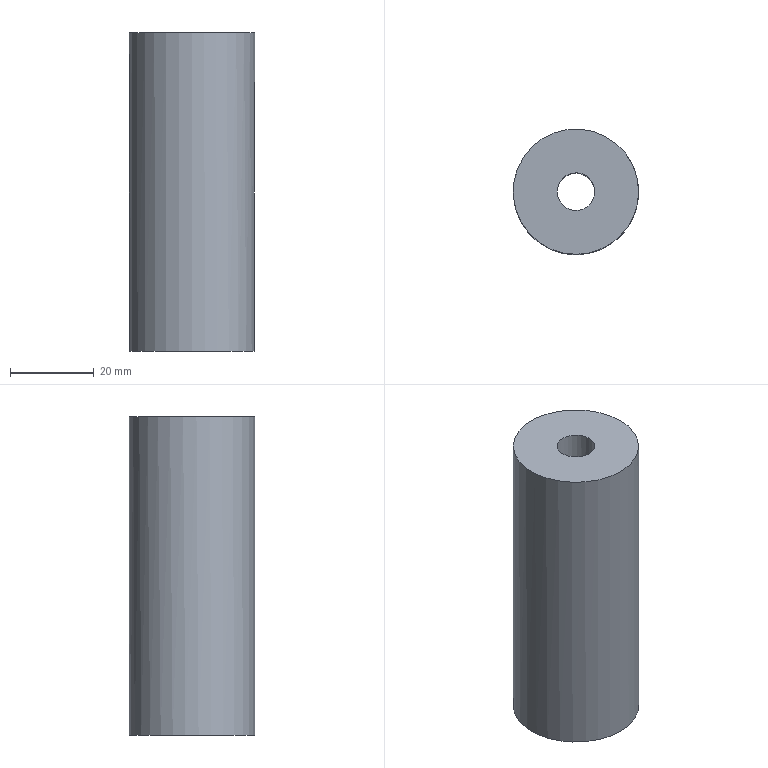Part | NX | features solid 2 | 1 solid | 6 faces | box 30 x 30 x 76.131 mm | volume 47845 mm3 | plane 3 | cylinder 3 | commonest cylinder face diameters 9.007 x1 14.508 x1 30 x1
STEP:
#1=CARTESIAN_POINT('',(797.773,-144.91,104.999));
#2=VERTEX_POINT('',#1);
#3=CARTESIAN_POINT('',(797.773,-129.91,104.999));
#4=DIRECTION('',(-0.000000328,0.000000403,-1.));
#5=DIRECTION('',(0.,-1.,-0.000000403));
#6=AXIS2_PLACEMENT_3D('',#3,#4,#5);
#7=CIRCLE('',#6,15.);
#8=EDGE_CURVE('',#2,#2,#7,.F.);
#9=ORIENTED_EDGE('',*,*,#8,.F.);
#10=EDGE_LOOP('',(#9));
#11=FACE_BOUND('',#10,.T.);
#12=CARTESIAN_POINT('',(796.295,-137.012,104.999));
#13=VERTEX_POINT('',#12);
#14=CARTESIAN_POINT('',(797.773,-129.91,104.999));
#15=DIRECTION('',(-0.000000328,0.000000403,-1.));
#16=DIRECTION('',(-0.2037,-0.979,-0.000000328));
#17=AXIS2_PLACEMENT_3D('',#14,#15,#16);
#18=CIRCLE('',#17,7.254);
#19=EDGE_CURVE('',#13,#13,#18,.F.);
#20=ORIENTED_EDGE('',*,*,#19,.T.);
#21=EDGE_LOOP('',(#20));
#22=FACE_BOUND('',#21,.T.);
#23=CARTESIAN_POINT('',(801.839,-133.976,104.999));
#24=DIRECTION('',(0.000000328,-0.000000403,1.));
#25=DIRECTION('',(-0.7071,-0.7071,-0.000000053));
#26=AXIS2_PLACEMENT_3D('',#23,#24,#25);
#27=PLANE('',#26);
#28=ADVANCED_FACE('',(#11,#22),#27,.F.);
#29=CARTESIAN_POINT('',(812.773,-129.91,181.13));
#30=VERTEX_POINT('',#29);
#31=CARTESIAN_POINT('',(797.773,-129.91,181.13));
#32=DIRECTION('',(0.,0.,-1.));
#33=DIRECTION('',(1.,0.,0.));
#34=AXIS2_PLACEMENT_3D('',#31,#32,#33);
#35=CIRCLE('',#34,15.);
#36=EDGE_CURVE('',#30,#30,#35,.F.);
#37=ORIENTED_EDGE('',*,*,#36,.F.);
#38=EDGE_LOOP('',(#37));
#39=FACE_BOUND('',#38,.T.);
#40=ORIENTED_EDGE('',*,*,#8,.T.);
#41=EDGE_LOOP('',(#40));
#42=FACE_BOUND('',#41,.T.);
#43=CARTESIAN_POINT('',(797.773,-129.91,96.999));
#44=DIRECTION('',(0.000000328,-0.000000403,1.));
#45=DIRECTION('',(-0.2037,-0.979,-0.000000328));
#46=AXIS2_PLACEMENT_3D('',#43,#44,#45);
#47=CYLINDRICAL_SURFACE('',#46,15.);
#48=ADVANCED_FACE('',(#39,#42),#47,.T.);
#49=CARTESIAN_POINT('',(802.276,-129.91,181.13));
#50=VERTEX_POINT('',#49);
#51=CARTESIAN_POINT('',(797.773,-129.91,181.13));
#52=DIRECTION('',(0.,0.,-1.));
#53=DIRECTION('',(1.,0.,0.));
#54=AXIS2_PLACEMENT_3D('',#51,#52,#53);
#55=CIRCLE('',#54,4.503);
#56=EDGE_CURVE('',#50,#50,#55,.T.);
#57=ORIENTED_EDGE('',*,*,#56,.T.);
#58=EDGE_LOOP('',(#57));
#59=FACE_BOUND('',#58,.T.);
#60=ORIENTED_EDGE('',*,*,#36,.T.);
#61=EDGE_LOOP('',(#60));
#62=FACE_BOUND('',#61,.T.);
#63=CARTESIAN_POINT('',(1379.977,36.59,181.13));
#64=DIRECTION('',(0.,0.,-1.));
#65=DIRECTION('',(0.,-1.,0.));
#66=AXIS2_PLACEMENT_3D('',#63,#64,#65);
#67=PLANE('',#66);
#68=ADVANCED_FACE('',(#59,#62),#67,.F.);
#69=CARTESIAN_POINT('',(797.773,-134.413,115.999));
#70=VERTEX_POINT('',#69);
#71=CARTESIAN_POINT('',(797.773,-129.91,115.999));
#72=DIRECTION('',(-0.000000328,0.000000403,-1.));
#73=DIRECTION('',(0.,-1.,-0.000000403));
#74=AXIS2_PLACEMENT_3D('',#71,#72,#73);
#75=CIRCLE('',#74,4.503);
#76=EDGE_CURVE('',#70,#70,#75,.F.);
#77=ORIENTED_EDGE('',*,*,#76,.F.);
#78=EDGE_LOOP('',(#77));
#79=FACE_BOUND('',#78,.T.);
#80=ORIENTED_EDGE('',*,*,#56,.F.);
#81=EDGE_LOOP('',(#80));
#82=FACE_BOUND('',#81,.T.);
#83=CARTESIAN_POINT('',(797.773,-129.91,104.999));
#84=DIRECTION('',(0.000000328,-0.000000403,1.));
#85=DIRECTION('',(-0.2037,-0.979,-0.000000328));
#86=AXIS2_PLACEMENT_3D('',#83,#84,#85);
#87=CYLINDRICAL_SURFACE('',#86,4.503);
#88=ADVANCED_FACE('',(#79,#82),#87,.F.);
#89=ORIENTED_EDGE('',*,*,#76,.T.);
#90=EDGE_LOOP('',(#89));
#91=FACE_BOUND('',#90,.T.);
#92=CARTESIAN_POINT('',(796.295,-137.012,115.999));
#93=VERTEX_POINT('',#92);
#94=CARTESIAN_POINT('',(797.773,-129.91,115.999));
#95=DIRECTION('',(0.000000328,-0.000000403,1.));
#96=DIRECTION('',(-0.2037,-0.979,-0.000000328));
#97=AXIS2_PLACEMENT_3D('',#94,#95,#96);
#98=CIRCLE('',#97,7.254);
#99=EDGE_CURVE('',#93,#93,#98,.T.);
#100=ORIENTED_EDGE('',*,*,#99,.F.);
#101=EDGE_LOOP('',(#100));
#102=FACE_BOUND('',#101,.T.);
#103=CARTESIAN_POINT('',(797.773,-129.91,115.999));
#104=DIRECTION('',(0.000000328,-0.000000403,1.));
#105=DIRECTION('',(0.,-1.,-0.000000403));
#106=AXIS2_PLACEMENT_3D('',#103,#104,#105);
#107=PLANE('',#106);
#108=ADVANCED_FACE('',(#91,#102),#107,.F.);
#109=ORIENTED_EDGE('',*,*,#99,.T.);
#110=EDGE_LOOP('',(#109));
#111=FACE_BOUND('',#110,.T.);
#112=ORIENTED_EDGE('',*,*,#19,.F.);
#113=EDGE_LOOP('',(#112));
#114=FACE_BOUND('',#113,.T.);
#115=CARTESIAN_POINT('',(797.773,-129.91,104.999));
#116=DIRECTION('',(0.000000328,-0.000000403,1.));
#117=DIRECTION('',(-0.2037,-0.979,-0.000000328));
#118=AXIS2_PLACEMENT_3D('',#115,#116,#117);
#119=CYLINDRICAL_SURFACE('',#118,7.254);
#120=ADVANCED_FACE('',(#111,#114),#119,.F.);
#121=CLOSED_SHELL('',(#28,#48,#68,#88,#108,#120));
#122=MANIFOLD_SOLID_BREP('',#121);
#123=(LENGTH_UNIT()NAMED_UNIT(*)SI_UNIT(.MILLI.,.METRE.));
#124=UNCERTAINTY_MEASURE_WITH_UNIT(LENGTH_MEASURE(0.00001),#123,'','');
#125=(NAMED_UNIT(*)PLANE_ANGLE_UNIT()SI_UNIT($,.RADIAN.));
#126=(NAMED_UNIT(*)SI_UNIT($,.STERADIAN.)SOLID_ANGLE_UNIT());
#127=(GEOMETRIC_REPRESENTATION_CONTEXT(3)GLOBAL_UNCERTAINTY_ASSIGNED_CONTEXT((#124))GLOBAL_UNIT_ASSIGNED_CONTEXT((#123,#125,#126))REPRESENTATION_CONTEXT('',''));
#128=ADVANCED_BREP_SHAPE_REPRESENTATION('',(#122),#127);